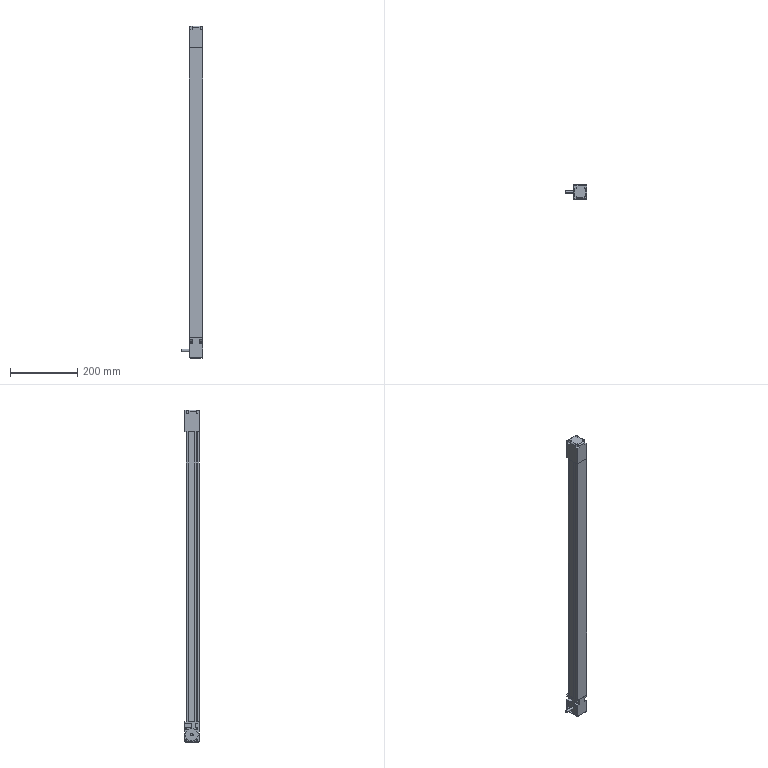Part | SolidWorks | features Cut 3, Boss 2, Fillet 2, ICE 2, Chamfer 1, Extrusion 1, HoleWzd 1 | 1 solid | 122 faces | box 64.5 x 44.058 x 985 mm | volume 1412008 mm3 | plane 82 | cylinder 30 | cone 10 | commonest cylinder face diameters 8 x16 3.3 x8 4 x4 37 x2